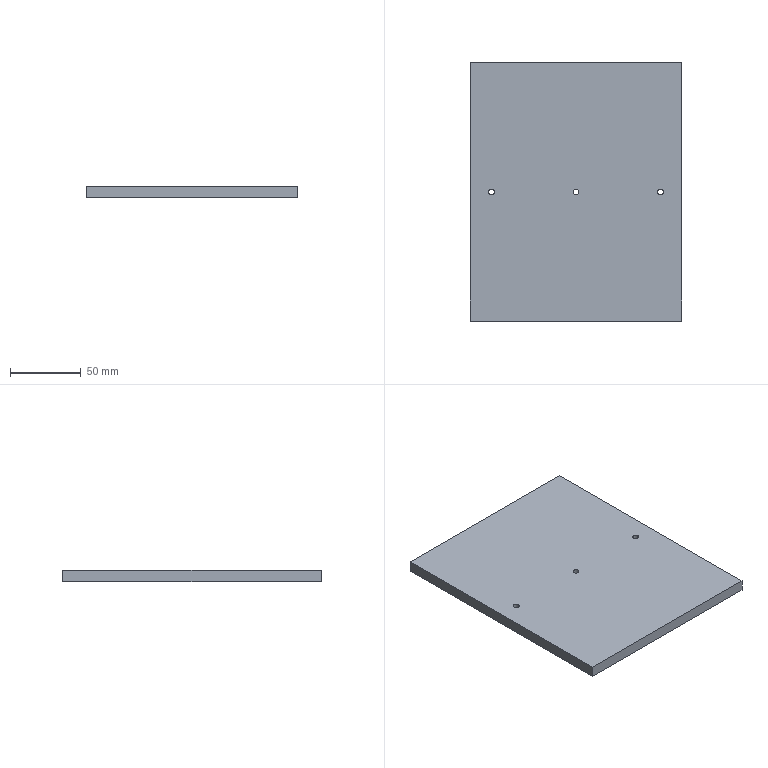Part | SolidWorks | features Extrusion 1, HoleWzd 1 | 1 solid | 12 faces | box 150 x 183 x 8 mm | volume 219267 mm3 | cylinder 6 | plane 6 | commonest cylinder face diameters 4.2 x6
STEP:
#1=CARTESIAN_POINT('',(-62.1,0.,-4.));
#2=VERTEX_POINT('',#1);
#3=CARTESIAN_POINT('',(-57.9,0.,-4.));
#4=VERTEX_POINT('',#3);
#5=CARTESIAN_POINT('',(-60.,0.,-4.));
#6=DIRECTION('',(0.,0.,1.));
#7=DIRECTION('',(1.,0.,0.));
#8=AXIS2_PLACEMENT_3D('',#5,#6,#7);
#9=CIRCLE('',#8,2.1);
#10=EDGE_CURVE('',#2,#4,#9,.T.);
#11=ORIENTED_EDGE('',*,*,#10,.F.);
#12=CARTESIAN_POINT('',(-62.1,0.,4.));
#13=VERTEX_POINT('',#12);
#14=CARTESIAN_POINT('',(-62.1,0.,4.));
#15=DIRECTION('',(0.,0.,1.));
#16=VECTOR('',#15,1000.);
#17=LINE('',#14,#16);
#18=EDGE_CURVE('',#2,#13,#17,.T.);
#19=ORIENTED_EDGE('',*,*,#18,.T.);
#20=CARTESIAN_POINT('',(-57.9,0.,4.));
#21=VERTEX_POINT('',#20);
#22=CARTESIAN_POINT('',(-60.,0.,4.));
#23=DIRECTION('',(0.,0.,1.));
#24=DIRECTION('',(1.,0.,0.));
#25=AXIS2_PLACEMENT_3D('',#22,#23,#24);
#26=CIRCLE('',#25,2.1);
#27=EDGE_CURVE('',#13,#21,#26,.T.);
#28=ORIENTED_EDGE('',*,*,#27,.T.);
#29=CARTESIAN_POINT('',(-57.9,0.,4.));
#30=DIRECTION('',(0.,0.,1.));
#31=VECTOR('',#30,1000.);
#32=LINE('',#29,#31);
#33=EDGE_CURVE('',#4,#21,#32,.T.);
#34=ORIENTED_EDGE('',*,*,#33,.F.);
#35=EDGE_LOOP('',(#11,#19,#28,#34));
#36=FACE_OUTER_BOUND('',#35,.T.);
#37=CARTESIAN_POINT('',(-60.,0.,4.));
#38=DIRECTION('',(0.,0.,1.));
#39=DIRECTION('',(1.,0.,0.));
#40=AXIS2_PLACEMENT_3D('',#37,#38,#39);
#41=CYLINDRICAL_SURFACE('',#40,2.1);
#42=ADVANCED_FACE('',(#36),#41,.F.);
#43=CARTESIAN_POINT('',(-2.1,0.,-4.));
#44=VERTEX_POINT('',#43);
#45=CARTESIAN_POINT('',(2.1,0.,-4.));
#46=VERTEX_POINT('',#45);
#47=CARTESIAN_POINT('',(0.,0.,-4.));
#48=DIRECTION('',(0.,0.,1.));
#49=DIRECTION('',(1.,0.,0.));
#50=AXIS2_PLACEMENT_3D('',#47,#48,#49);
#51=CIRCLE('',#50,2.1);
#52=EDGE_CURVE('',#44,#46,#51,.T.);
#53=ORIENTED_EDGE('',*,*,#52,.F.);
#54=CARTESIAN_POINT('',(-2.1,0.,4.));
#55=VERTEX_POINT('',#54);
#56=CARTESIAN_POINT('',(-2.1,0.,4.));
#57=DIRECTION('',(0.,0.,1.));
#58=VECTOR('',#57,1000.);
#59=LINE('',#56,#58);
#60=EDGE_CURVE('',#44,#55,#59,.T.);
#61=ORIENTED_EDGE('',*,*,#60,.T.);
#62=CARTESIAN_POINT('',(2.1,0.,4.));
#63=VERTEX_POINT('',#62);
#64=CARTESIAN_POINT('',(0.,0.,4.));
#65=DIRECTION('',(0.,0.,1.));
#66=DIRECTION('',(1.,0.,0.));
#67=AXIS2_PLACEMENT_3D('',#64,#65,#66);
#68=CIRCLE('',#67,2.1);
#69=EDGE_CURVE('',#55,#63,#68,.T.);
#70=ORIENTED_EDGE('',*,*,#69,.T.);
#71=CARTESIAN_POINT('',(2.1,0.,4.));
#72=DIRECTION('',(0.,0.,1.));
#73=VECTOR('',#72,1000.);
#74=LINE('',#71,#73);
#75=EDGE_CURVE('',#46,#63,#74,.T.);
#76=ORIENTED_EDGE('',*,*,#75,.F.);
#77=EDGE_LOOP('',(#53,#61,#70,#76));
#78=FACE_OUTER_BOUND('',#77,.T.);
#79=CARTESIAN_POINT('',(0.,0.,4.));
#80=DIRECTION('',(0.,0.,1.));
#81=DIRECTION('',(1.,0.,0.));
#82=AXIS2_PLACEMENT_3D('',#79,#80,#81);
#83=CYLINDRICAL_SURFACE('',#82,2.1);
#84=ADVANCED_FACE('',(#78),#83,.F.);
#85=CARTESIAN_POINT('',(57.9,0.,-4.));
#86=VERTEX_POINT('',#85);
#87=CARTESIAN_POINT('',(62.1,0.,-4.));
#88=VERTEX_POINT('',#87);
#89=CARTESIAN_POINT('',(60.,0.,-4.));
#90=DIRECTION('',(0.,0.,1.));
#91=DIRECTION('',(1.,0.,0.));
#92=AXIS2_PLACEMENT_3D('',#89,#90,#91);
#93=CIRCLE('',#92,2.1);
#94=EDGE_CURVE('',#86,#88,#93,.T.);
#95=ORIENTED_EDGE('',*,*,#94,.F.);
#96=CARTESIAN_POINT('',(57.9,0.,4.));
#97=VERTEX_POINT('',#96);
#98=CARTESIAN_POINT('',(57.9,0.,4.));
#99=DIRECTION('',(0.,0.,1.));
#100=VECTOR('',#99,1000.);
#101=LINE('',#98,#100);
#102=EDGE_CURVE('',#86,#97,#101,.T.);
#103=ORIENTED_EDGE('',*,*,#102,.T.);
#104=CARTESIAN_POINT('',(62.1,0.,4.));
#105=VERTEX_POINT('',#104);
#106=CARTESIAN_POINT('',(60.,0.,4.));
#107=DIRECTION('',(0.,0.,1.));
#108=DIRECTION('',(1.,0.,0.));
#109=AXIS2_PLACEMENT_3D('',#106,#107,#108);
#110=CIRCLE('',#109,2.1);
#111=EDGE_CURVE('',#97,#105,#110,.T.);
#112=ORIENTED_EDGE('',*,*,#111,.T.);
#113=CARTESIAN_POINT('',(62.1,0.,4.));
#114=DIRECTION('',(0.,0.,1.));
#115=VECTOR('',#114,1000.);
#116=LINE('',#113,#115);
#117=EDGE_CURVE('',#88,#105,#116,.T.);
#118=ORIENTED_EDGE('',*,*,#117,.F.);
#119=EDGE_LOOP('',(#95,#103,#112,#118));
#120=FACE_OUTER_BOUND('',#119,.T.);
#121=CARTESIAN_POINT('',(60.,0.,4.));
#122=DIRECTION('',(0.,0.,1.));
#123=DIRECTION('',(1.,0.,0.));
#124=AXIS2_PLACEMENT_3D('',#121,#122,#123);
#125=CYLINDRICAL_SURFACE('',#124,2.1);
#126=ADVANCED_FACE('',(#120),#125,.F.);
#127=CARTESIAN_POINT('',(-75.,91.5,-4.));
#128=VERTEX_POINT('',#127);
#129=CARTESIAN_POINT('',(-75.,-91.5,-4.));
#130=VERTEX_POINT('',#129);
#131=CARTESIAN_POINT('',(-75.,-91.5,-4.));
#132=DIRECTION('',(0.,-1.,0.));
#133=VECTOR('',#132,1000.);
#134=LINE('',#131,#133);
#135=EDGE_CURVE('',#128,#130,#134,.T.);
#136=ORIENTED_EDGE('',*,*,#135,.T.);
#137=CARTESIAN_POINT('',(-75.,-91.5,4.));
#138=VERTEX_POINT('',#137);
#139=CARTESIAN_POINT('',(-75.,-91.5,4.));
#140=DIRECTION('',(0.,0.,-1.));
#141=VECTOR('',#140,1000.);
#142=LINE('',#139,#141);
#143=EDGE_CURVE('',#138,#130,#142,.T.);
#144=ORIENTED_EDGE('',*,*,#143,.F.);
#145=CARTESIAN_POINT('',(-75.,91.5,4.));
#146=VERTEX_POINT('',#145);
#147=CARTESIAN_POINT('',(-75.,-91.5,4.));
#148=DIRECTION('',(0.,-1.,0.));
#149=VECTOR('',#148,1000.);
#150=LINE('',#147,#149);
#151=EDGE_CURVE('',#146,#138,#150,.T.);
#152=ORIENTED_EDGE('',*,*,#151,.F.);
#153=CARTESIAN_POINT('',(-75.,91.5,4.));
#154=DIRECTION('',(0.,0.,-1.));
#155=VECTOR('',#154,1000.);
#156=LINE('',#153,#155);
#157=EDGE_CURVE('',#146,#128,#156,.T.);
#158=ORIENTED_EDGE('',*,*,#157,.T.);
#159=EDGE_LOOP('',(#136,#144,#152,#158));
#160=FACE_OUTER_BOUND('',#159,.T.);
#161=CARTESIAN_POINT('',(-75.,-91.5,4.));
#162=DIRECTION('',(1.,0.,0.));
#163=DIRECTION('',(0.,0.,-1.));
#164=AXIS2_PLACEMENT_3D('',#161,#162,#163);
#165=PLANE('',#164);
#166=ADVANCED_FACE('',(#160),#165,.F.);
#167=CARTESIAN_POINT('',(75.,-91.5,-4.));
#168=VERTEX_POINT('',#167);
#169=CARTESIAN_POINT('',(75.,-91.5,-4.));
#170=DIRECTION('',(1.,0.,0.));
#171=VECTOR('',#170,1000.);
#172=LINE('',#169,#171);
#173=EDGE_CURVE('',#130,#168,#172,.T.);
#174=ORIENTED_EDGE('',*,*,#173,.T.);
#175=CARTESIAN_POINT('',(75.,-91.5,4.));
#176=VERTEX_POINT('',#175);
#177=CARTESIAN_POINT('',(75.,-91.5,4.));
#178=DIRECTION('',(0.,0.,-1.));
#179=VECTOR('',#178,1000.);
#180=LINE('',#177,#179);
#181=EDGE_CURVE('',#176,#168,#180,.T.);
#182=ORIENTED_EDGE('',*,*,#181,.F.);
#183=CARTESIAN_POINT('',(75.,-91.5,4.));
#184=DIRECTION('',(1.,0.,0.));
#185=VECTOR('',#184,1000.);
#186=LINE('',#183,#185);
#187=EDGE_CURVE('',#138,#176,#186,.T.);
#188=ORIENTED_EDGE('',*,*,#187,.F.);
#189=ORIENTED_EDGE('',*,*,#143,.T.);
#190=EDGE_LOOP('',(#174,#182,#188,#189));
#191=FACE_OUTER_BOUND('',#190,.T.);
#192=CARTESIAN_POINT('',(75.,-91.5,4.));
#193=DIRECTION('',(0.,1.,0.));
#194=DIRECTION('',(-1.,0.,0.));
#195=AXIS2_PLACEMENT_3D('',#192,#193,#194);
#196=PLANE('',#195);
#197=ADVANCED_FACE('',(#191),#196,.F.);
#198=CARTESIAN_POINT('',(75.,91.5,-4.));
#199=VERTEX_POINT('',#198);
#200=CARTESIAN_POINT('',(75.,-91.5,-4.));
#201=DIRECTION('',(0.,1.,0.));
#202=VECTOR('',#201,1000.);
#203=LINE('',#200,#202);
#204=EDGE_CURVE('',#168,#199,#203,.T.);
#205=ORIENTED_EDGE('',*,*,#204,.T.);
#206=CARTESIAN_POINT('',(75.,91.5,4.));
#207=VERTEX_POINT('',#206);
#208=CARTESIAN_POINT('',(75.,91.5,4.));
#209=DIRECTION('',(0.,0.,-1.));
#210=VECTOR('',#209,1000.);
#211=LINE('',#208,#210);
#212=EDGE_CURVE('',#207,#199,#211,.T.);
#213=ORIENTED_EDGE('',*,*,#212,.F.);
#214=CARTESIAN_POINT('',(75.,-91.5,4.));
#215=DIRECTION('',(0.,1.,0.));
#216=VECTOR('',#215,1000.);
#217=LINE('',#214,#216);
#218=EDGE_CURVE('',#176,#207,#217,.T.);
#219=ORIENTED_EDGE('',*,*,#218,.F.);
#220=ORIENTED_EDGE('',*,*,#181,.T.);
#221=EDGE_LOOP('',(#205,#213,#219,#220));
#222=FACE_OUTER_BOUND('',#221,.T.);
#223=CARTESIAN_POINT('',(75.,-91.5,4.));
#224=DIRECTION('',(-1.,0.,0.));
#225=DIRECTION('',(0.,0.,1.));
#226=AXIS2_PLACEMENT_3D('',#223,#224,#225);
#227=PLANE('',#226);
#228=ADVANCED_FACE('',(#222),#227,.F.);
#229=CARTESIAN_POINT('',(75.,91.5,-4.));
#230=DIRECTION('',(-1.,0.,0.));
#231=VECTOR('',#230,1000.);
#232=LINE('',#229,#231);
#233=EDGE_CURVE('',#199,#128,#232,.T.);
#234=ORIENTED_EDGE('',*,*,#233,.T.);
#235=ORIENTED_EDGE('',*,*,#157,.F.);
#236=CARTESIAN_POINT('',(75.,91.5,4.));
#237=DIRECTION('',(-1.,0.,0.));
#238=VECTOR('',#237,1000.);
#239=LINE('',#236,#238);
#240=EDGE_CURVE('',#207,#146,#239,.T.);
#241=ORIENTED_EDGE('',*,*,#240,.F.);
#242=ORIENTED_EDGE('',*,*,#212,.T.);
#243=EDGE_LOOP('',(#234,#235,#241,#242));
#244=FACE_OUTER_BOUND('',#243,.T.);
#245=CARTESIAN_POINT('',(75.,91.5,4.));
#246=DIRECTION('',(0.,-1.,0.));
#247=DIRECTION('',(0.,0.,-1.));
#248=AXIS2_PLACEMENT_3D('',#245,#246,#247);
#249=PLANE('',#248);
#250=ADVANCED_FACE('',(#244),#249,.F.);
#251=CARTESIAN_POINT('',(-60.,0.,4.));
#252=DIRECTION('',(0.,0.,1.));
#253=DIRECTION('',(1.,0.,0.));
#254=AXIS2_PLACEMENT_3D('',#251,#252,#253);
#255=CIRCLE('',#254,2.1);
#256=EDGE_CURVE('',#21,#13,#255,.T.);
#257=ORIENTED_EDGE('',*,*,#256,.F.);
#258=ORIENTED_EDGE('',*,*,#27,.F.);
#259=EDGE_LOOP('',(#257,#258));
#260=FACE_BOUND('',#259,.T.);
#261=CARTESIAN_POINT('',(0.,0.,4.));
#262=DIRECTION('',(0.,0.,1.));
#263=DIRECTION('',(1.,0.,0.));
#264=AXIS2_PLACEMENT_3D('',#261,#262,#263);
#265=CIRCLE('',#264,2.1);
#266=EDGE_CURVE('',#63,#55,#265,.T.);
#267=ORIENTED_EDGE('',*,*,#266,.F.);
#268=ORIENTED_EDGE('',*,*,#69,.F.);
#269=EDGE_LOOP('',(#267,#268));
#270=FACE_BOUND('',#269,.T.);
#271=CARTESIAN_POINT('',(60.,0.,4.));
#272=DIRECTION('',(0.,0.,1.));
#273=DIRECTION('',(1.,0.,0.));
#274=AXIS2_PLACEMENT_3D('',#271,#272,#273);
#275=CIRCLE('',#274,2.1);
#276=EDGE_CURVE('',#105,#97,#275,.T.);
#277=ORIENTED_EDGE('',*,*,#276,.F.);
#278=ORIENTED_EDGE('',*,*,#111,.F.);
#279=EDGE_LOOP('',(#277,#278));
#280=FACE_BOUND('',#279,.T.);
#281=ORIENTED_EDGE('',*,*,#151,.T.);
#282=ORIENTED_EDGE('',*,*,#187,.T.);
#283=ORIENTED_EDGE('',*,*,#218,.T.);
#284=ORIENTED_EDGE('',*,*,#240,.T.);
#285=EDGE_LOOP('',(#281,#282,#283,#284));
#286=FACE_OUTER_BOUND('',#285,.T.);
#287=CARTESIAN_POINT('',(0.,0.,4.));
#288=DIRECTION('',(0.,0.,1.));
#289=DIRECTION('',(1.,0.,0.));
#290=AXIS2_PLACEMENT_3D('',#287,#288,#289);
#291=PLANE('',#290);
#292=ADVANCED_FACE('',(#260,#270,#280,#286),#291,.T.);
#293=CARTESIAN_POINT('',(-60.,0.,-4.));
#294=DIRECTION('',(0.,0.,1.));
#295=DIRECTION('',(1.,0.,0.));
#296=AXIS2_PLACEMENT_3D('',#293,#294,#295);
#297=CIRCLE('',#296,2.1);
#298=EDGE_CURVE('',#4,#2,#297,.T.);
#299=ORIENTED_EDGE('',*,*,#298,.T.);
#300=ORIENTED_EDGE('',*,*,#10,.T.);
#301=EDGE_LOOP('',(#299,#300));
#302=FACE_BOUND('',#301,.T.);
#303=CARTESIAN_POINT('',(0.,0.,-4.));
#304=DIRECTION('',(0.,0.,1.));
#305=DIRECTION('',(1.,0.,0.));
#306=AXIS2_PLACEMENT_3D('',#303,#304,#305);
#307=CIRCLE('',#306,2.1);
#308=EDGE_CURVE('',#46,#44,#307,.T.);
#309=ORIENTED_EDGE('',*,*,#308,.T.);
#310=ORIENTED_EDGE('',*,*,#52,.T.);
#311=EDGE_LOOP('',(#309,#310));
#312=FACE_BOUND('',#311,.T.);
#313=CARTESIAN_POINT('',(60.,0.,-4.));
#314=DIRECTION('',(0.,0.,1.));
#315=DIRECTION('',(1.,0.,0.));
#316=AXIS2_PLACEMENT_3D('',#313,#314,#315);
#317=CIRCLE('',#316,2.1);
#318=EDGE_CURVE('',#88,#86,#317,.T.);
#319=ORIENTED_EDGE('',*,*,#318,.T.);
#320=ORIENTED_EDGE('',*,*,#94,.T.);
#321=EDGE_LOOP('',(#319,#320));
#322=FACE_BOUND('',#321,.T.);
#323=ORIENTED_EDGE('',*,*,#135,.F.);
#324=ORIENTED_EDGE('',*,*,#233,.F.);
#325=ORIENTED_EDGE('',*,*,#204,.F.);
#326=ORIENTED_EDGE('',*,*,#173,.F.);
#327=EDGE_LOOP('',(#323,#324,#325,#326));
#328=FACE_OUTER_BOUND('',#327,.T.);
#329=CARTESIAN_POINT('',(0.,0.,-4.));
#330=DIRECTION('',(0.,0.,1.));
#331=DIRECTION('',(1.,0.,0.));
#332=AXIS2_PLACEMENT_3D('',#329,#330,#331);
#333=PLANE('',#332);
#334=ADVANCED_FACE('',(#302,#312,#322,#328),#333,.F.);
#335=ORIENTED_EDGE('',*,*,#102,.F.);
#336=ORIENTED_EDGE('',*,*,#318,.F.);
#337=ORIENTED_EDGE('',*,*,#117,.T.);
#338=ORIENTED_EDGE('',*,*,#276,.T.);
#339=EDGE_LOOP('',(#335,#336,#337,#338));
#340=FACE_OUTER_BOUND('',#339,.T.);
#341=CARTESIAN_POINT('',(60.,0.,4.));
#342=DIRECTION('',(0.,0.,1.));
#343=DIRECTION('',(1.,0.,0.));
#344=AXIS2_PLACEMENT_3D('',#341,#342,#343);
#345=CYLINDRICAL_SURFACE('',#344,2.1);
#346=ADVANCED_FACE('',(#340),#345,.F.);
#347=ORIENTED_EDGE('',*,*,#60,.F.);
#348=ORIENTED_EDGE('',*,*,#308,.F.);
#349=ORIENTED_EDGE('',*,*,#75,.T.);
#350=ORIENTED_EDGE('',*,*,#266,.T.);
#351=EDGE_LOOP('',(#347,#348,#349,#350));
#352=FACE_OUTER_BOUND('',#351,.T.);
#353=CARTESIAN_POINT('',(0.,0.,4.));
#354=DIRECTION('',(0.,0.,1.));
#355=DIRECTION('',(1.,0.,0.));
#356=AXIS2_PLACEMENT_3D('',#353,#354,#355);
#357=CYLINDRICAL_SURFACE('',#356,2.1);
#358=ADVANCED_FACE('',(#352),#357,.F.);
#359=ORIENTED_EDGE('',*,*,#18,.F.);
#360=ORIENTED_EDGE('',*,*,#298,.F.);
#361=ORIENTED_EDGE('',*,*,#33,.T.);
#362=ORIENTED_EDGE('',*,*,#256,.T.);
#363=EDGE_LOOP('',(#359,#360,#361,#362));
#364=FACE_OUTER_BOUND('',#363,.T.);
#365=CARTESIAN_POINT('',(-60.,0.,4.));
#366=DIRECTION('',(0.,0.,1.));
#367=DIRECTION('',(1.,0.,0.));
#368=AXIS2_PLACEMENT_3D('',#365,#366,#367);
#369=CYLINDRICAL_SURFACE('',#368,2.1);
#370=ADVANCED_FACE('',(#364),#369,.F.);
#371=CLOSED_SHELL('',(#42,#84,#126,#166,#197,#228,#250,#292,#334,#346,#358,#370));
#372=MANIFOLD_SOLID_BREP('',#371);
#373=CARTESIAN_POINT('',(0.,0.,0.));
#374=DIRECTION('',(0.,0.,1.));
#375=DIRECTION('',(1.,0.,0.));
#376=AXIS2_PLACEMENT_3D('',#373,#374,#375);
#377=(LENGTH_UNIT()NAMED_UNIT(*)SI_UNIT(.MILLI.,.METRE.));
#378=UNCERTAINTY_MEASURE_WITH_UNIT(LENGTH_MEASURE(0.00001),#377,'','');
#379=(NAMED_UNIT(*)PLANE_ANGLE_UNIT()SI_UNIT($,.RADIAN.));
#380=(NAMED_UNIT(*)SI_UNIT($,.STERADIAN.)SOLID_ANGLE_UNIT());
#381=(GEOMETRIC_REPRESENTATION_CONTEXT(3)GLOBAL_UNCERTAINTY_ASSIGNED_CONTEXT((#378))GLOBAL_UNIT_ASSIGNED_CONTEXT((#377,#379,#380))REPRESENTATION_CONTEXT('',''));
#382=ADVANCED_BREP_SHAPE_REPRESENTATION('',(#372,#376),#381);